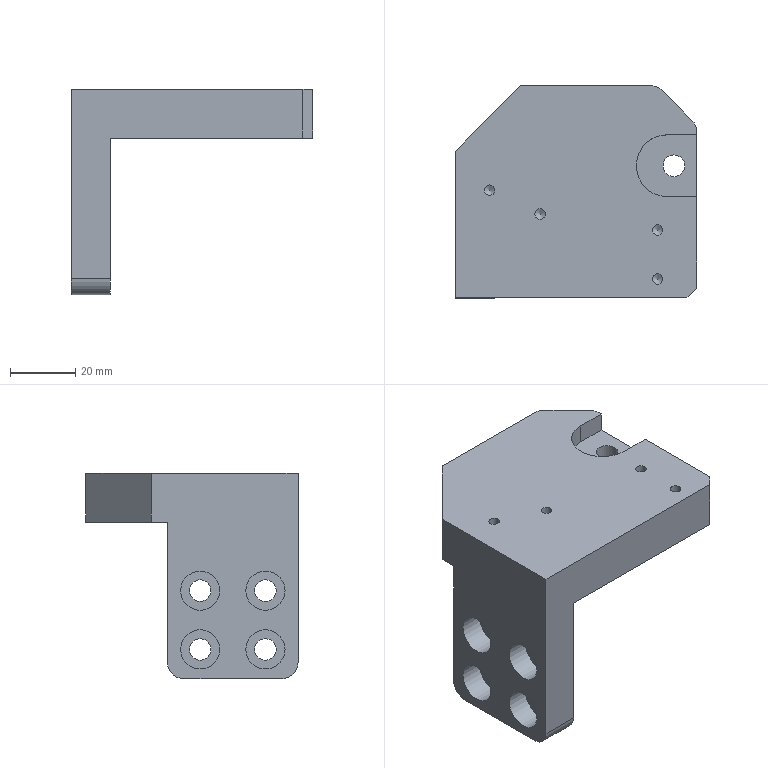Part | NX | 1 solid | 41 faces | box 74 x 65 x 63 mm | volume 84454 mm3 | plane 19 | cylinder 18 | cone 4 | commonest cylinder face diameters 3.242 x4 6.6 x4 10 x4 12 x4 6.647 x1 19 x1
STEP:
#1=CARTESIAN_POINT('',(-29.8,-5.8,-36.));
#2=VERTEX_POINT('',#1);
#3=CARTESIAN_POINT('',(-29.8,-2.5,-36.));
#4=DIRECTION('',(1.,0.,0.));
#5=DIRECTION('',(0.,-1.,0.));
#6=AXIS2_PLACEMENT_3D('',#3,#4,#5);
#7=CIRCLE('',#6,3.3);
#8=EDGE_CURVE('',#2,#2,#7,.T.);
#9=ORIENTED_EDGE('',*,*,#8,.T.);
#10=EDGE_LOOP('',(#9));
#11=FACE_BOUND('',#10,.T.);
#12=CARTESIAN_POINT('',(-29.8,-8.5,-36.));
#13=VERTEX_POINT('',#12);
#14=CARTESIAN_POINT('',(-29.8,-2.5,-36.));
#15=DIRECTION('',(-1.,0.,0.));
#16=DIRECTION('',(0.,-1.,0.));
#17=AXIS2_PLACEMENT_3D('',#14,#15,#16);
#18=CIRCLE('',#17,6.);
#19=EDGE_CURVE('',#13,#13,#18,.T.);
#20=ORIENTED_EDGE('',*,*,#19,.T.);
#21=EDGE_LOOP('',(#20));
#22=FACE_BOUND('',#21,.T.);
#23=CARTESIAN_POINT('',(-29.8,32.5,0.));
#24=DIRECTION('',(-1.,0.,0.));
#25=DIRECTION('',(0.,-1.,0.));
#26=AXIS2_PLACEMENT_3D('',#23,#24,#25);
#27=PLANE('',#26);
#28=ADVANCED_FACE('',(#11,#22),#27,.T.);
#29=CARTESIAN_POINT('',(-37.,-8.5,-36.));
#30=VERTEX_POINT('',#29);
#31=CARTESIAN_POINT('',(-37.,-2.5,-36.));
#32=DIRECTION('',(-1.,0.,0.));
#33=DIRECTION('',(0.,-1.,0.));
#34=AXIS2_PLACEMENT_3D('',#31,#32,#33);
#35=CIRCLE('',#34,6.);
#36=EDGE_CURVE('',#30,#30,#35,.T.);
#37=ORIENTED_EDGE('',*,*,#36,.T.);
#38=EDGE_LOOP('',(#37));
#39=FACE_BOUND('',#38,.T.);
#40=ORIENTED_EDGE('',*,*,#19,.F.);
#41=EDGE_LOOP('',(#40));
#42=FACE_BOUND('',#41,.T.);
#43=CARTESIAN_POINT('',(-33.4,-2.5,-36.));
#44=DIRECTION('',(-1.,0.,0.));
#45=DIRECTION('',(0.,-1.,0.));
#46=AXIS2_PLACEMENT_3D('',#43,#44,#45);
#47=CYLINDRICAL_SURFACE('',#46,6.);
#48=ADVANCED_FACE('',(#39,#42),#47,.F.);
#49=CARTESIAN_POINT('',(-29.8,-5.8,-54.));
#50=VERTEX_POINT('',#49);
#51=CARTESIAN_POINT('',(-29.8,-2.5,-54.));
#52=DIRECTION('',(1.,0.,0.));
#53=DIRECTION('',(0.,-1.,0.));
#54=AXIS2_PLACEMENT_3D('',#51,#52,#53);
#55=CIRCLE('',#54,3.3);
#56=EDGE_CURVE('',#50,#50,#55,.T.);
#57=ORIENTED_EDGE('',*,*,#56,.T.);
#58=EDGE_LOOP('',(#57));
#59=FACE_BOUND('',#58,.T.);
#60=CARTESIAN_POINT('',(-29.8,-8.5,-54.));
#61=VERTEX_POINT('',#60);
#62=CARTESIAN_POINT('',(-29.8,-2.5,-54.));
#63=DIRECTION('',(-1.,0.,0.));
#64=DIRECTION('',(0.,-1.,0.));
#65=AXIS2_PLACEMENT_3D('',#62,#63,#64);
#66=CIRCLE('',#65,6.);
#67=EDGE_CURVE('',#61,#61,#66,.T.);
#68=ORIENTED_EDGE('',*,*,#67,.T.);
#69=EDGE_LOOP('',(#68));
#70=FACE_BOUND('',#69,.T.);
#71=CARTESIAN_POINT('',(-29.8,32.5,0.));
#72=DIRECTION('',(-1.,0.,0.));
#73=DIRECTION('',(0.,-1.,0.));
#74=AXIS2_PLACEMENT_3D('',#71,#72,#73);
#75=PLANE('',#74);
#76=ADVANCED_FACE('',(#59,#70),#75,.T.);
#77=CARTESIAN_POINT('',(-37.,-8.5,-54.));
#78=VERTEX_POINT('',#77);
#79=CARTESIAN_POINT('',(-37.,-2.5,-54.));
#80=DIRECTION('',(-1.,0.,0.));
#81=DIRECTION('',(0.,-1.,0.));
#82=AXIS2_PLACEMENT_3D('',#79,#80,#81);
#83=CIRCLE('',#82,6.);
#84=EDGE_CURVE('',#78,#78,#83,.T.);
#85=ORIENTED_EDGE('',*,*,#84,.T.);
#86=EDGE_LOOP('',(#85));
#87=FACE_BOUND('',#86,.T.);
#88=ORIENTED_EDGE('',*,*,#67,.F.);
#89=EDGE_LOOP('',(#88));
#90=FACE_BOUND('',#89,.T.);
#91=CARTESIAN_POINT('',(-33.4,-2.5,-54.));
#92=DIRECTION('',(-1.,0.,0.));
#93=DIRECTION('',(0.,-1.,0.));
#94=AXIS2_PLACEMENT_3D('',#91,#92,#93);
#95=CYLINDRICAL_SURFACE('',#94,6.);
#96=ADVANCED_FACE('',(#87,#90),#95,.F.);
#97=CARTESIAN_POINT('',(-29.8,-25.8,-36.));
#98=VERTEX_POINT('',#97);
#99=CARTESIAN_POINT('',(-29.8,-22.5,-36.));
#100=DIRECTION('',(1.,0.,0.));
#101=DIRECTION('',(0.,-1.,0.));
#102=AXIS2_PLACEMENT_3D('',#99,#100,#101);
#103=CIRCLE('',#102,3.3);
#104=EDGE_CURVE('',#98,#98,#103,.T.);
#105=ORIENTED_EDGE('',*,*,#104,.T.);
#106=EDGE_LOOP('',(#105));
#107=FACE_BOUND('',#106,.T.);
#108=CARTESIAN_POINT('',(-29.8,-28.5,-36.));
#109=VERTEX_POINT('',#108);
#110=CARTESIAN_POINT('',(-29.8,-22.5,-36.));
#111=DIRECTION('',(-1.,0.,0.));
#112=DIRECTION('',(0.,-1.,0.));
#113=AXIS2_PLACEMENT_3D('',#110,#111,#112);
#114=CIRCLE('',#113,6.);
#115=EDGE_CURVE('',#109,#109,#114,.T.);
#116=ORIENTED_EDGE('',*,*,#115,.T.);
#117=EDGE_LOOP('',(#116));
#118=FACE_BOUND('',#117,.T.);
#119=CARTESIAN_POINT('',(-29.8,32.5,0.));
#120=DIRECTION('',(-1.,0.,0.));
#121=DIRECTION('',(0.,-1.,0.));
#122=AXIS2_PLACEMENT_3D('',#119,#120,#121);
#123=PLANE('',#122);
#124=ADVANCED_FACE('',(#107,#118),#123,.T.);
#125=CARTESIAN_POINT('',(-37.,-28.5,-36.));
#126=VERTEX_POINT('',#125);
#127=CARTESIAN_POINT('',(-37.,-22.5,-36.));
#128=DIRECTION('',(-1.,0.,0.));
#129=DIRECTION('',(0.,-1.,0.));
#130=AXIS2_PLACEMENT_3D('',#127,#128,#129);
#131=CIRCLE('',#130,6.);
#132=EDGE_CURVE('',#126,#126,#131,.T.);
#133=ORIENTED_EDGE('',*,*,#132,.T.);
#134=EDGE_LOOP('',(#133));
#135=FACE_BOUND('',#134,.T.);
#136=ORIENTED_EDGE('',*,*,#115,.F.);
#137=EDGE_LOOP('',(#136));
#138=FACE_BOUND('',#137,.T.);
#139=CARTESIAN_POINT('',(-33.4,-22.5,-36.));
#140=DIRECTION('',(-1.,0.,0.));
#141=DIRECTION('',(0.,-1.,0.));
#142=AXIS2_PLACEMENT_3D('',#139,#140,#141);
#143=CYLINDRICAL_SURFACE('',#142,6.);
#144=ADVANCED_FACE('',(#135,#138),#143,.F.);
#145=CARTESIAN_POINT('',(30.,4.676,-15.));
#146=VERTEX_POINT('',#145);
#147=CARTESIAN_POINT('',(30.,8.,-15.));
#148=DIRECTION('',(0.,0.,1.));
#149=DIRECTION('',(0.,-1.,0.));
#150=AXIS2_PLACEMENT_3D('',#147,#148,#149);
#151=CIRCLE('',#150,3.324);
#152=EDGE_CURVE('',#146,#146,#151,.T.);
#153=ORIENTED_EDGE('',*,*,#152,.F.);
#154=EDGE_LOOP('',(#153));
#155=FACE_BOUND('',#154,.T.);
#156=CARTESIAN_POINT('',(30.,4.676,-6.));
#157=VERTEX_POINT('',#156);
#158=CARTESIAN_POINT('',(30.,8.,-6.));
#159=DIRECTION('',(0.,0.,1.));
#160=DIRECTION('',(0.,-1.,0.));
#161=AXIS2_PLACEMENT_3D('',#158,#159,#160);
#162=CIRCLE('',#161,3.324);
#163=EDGE_CURVE('',#157,#157,#162,.T.);
#164=ORIENTED_EDGE('',*,*,#163,.T.);
#165=EDGE_LOOP('',(#164));
#166=FACE_BOUND('',#165,.T.);
#167=CARTESIAN_POINT('',(30.,8.,-6.));
#168=DIRECTION('',(0.,0.,-1.));
#169=DIRECTION('',(0.,-1.,0.));
#170=AXIS2_PLACEMENT_3D('',#167,#168,#169);
#171=CYLINDRICAL_SURFACE('',#170,3.324);
#172=ADVANCED_FACE('',(#155,#166),#171,.F.);
#173=CARTESIAN_POINT('',(-25.,-25.8,-54.));
#174=VERTEX_POINT('',#173);
#175=CARTESIAN_POINT('',(-25.,-22.5,-54.));
#176=DIRECTION('',(1.,0.,0.));
#177=DIRECTION('',(0.,-1.,0.));
#178=AXIS2_PLACEMENT_3D('',#175,#176,#177);
#179=CIRCLE('',#178,3.3);
#180=EDGE_CURVE('',#174,#174,#179,.T.);
#181=ORIENTED_EDGE('',*,*,#180,.T.);
#182=EDGE_LOOP('',(#181));
#183=FACE_BOUND('',#182,.T.);
#184=CARTESIAN_POINT('',(-29.8,-25.8,-54.));
#185=VERTEX_POINT('',#184);
#186=CARTESIAN_POINT('',(-29.8,-22.5,-54.));
#187=DIRECTION('',(-1.,0.,0.));
#188=DIRECTION('',(0.,-1.,0.));
#189=AXIS2_PLACEMENT_3D('',#186,#187,#188);
#190=CIRCLE('',#189,3.3);
#191=EDGE_CURVE('',#185,#185,#190,.T.);
#192=ORIENTED_EDGE('',*,*,#191,.T.);
#193=EDGE_LOOP('',(#192));
#194=FACE_BOUND('',#193,.T.);
#195=CARTESIAN_POINT('',(-57.5,-22.5,-54.));
#196=DIRECTION('',(1.,0.,0.));
#197=DIRECTION('',(0.,1.,0.));
#198=AXIS2_PLACEMENT_3D('',#195,#196,#197);
#199=CYLINDRICAL_SURFACE('',#198,3.3);
#200=ADVANCED_FACE('',(#183,#194),#199,.F.);
#201=CARTESIAN_POINT('',(-26.5,2.121,-10.));
#202=VERTEX_POINT('',#201);
#203=CARTESIAN_POINT('',(-26.5,0.5,-10.));
#204=DIRECTION('',(0.,0.,-1.));
#205=DIRECTION('',(0.,1.,0.));
#206=AXIS2_PLACEMENT_3D('',#203,#204,#205);
#207=CIRCLE('',#206,1.621);
#208=EDGE_CURVE('',#202,#202,#207,.T.);
#209=ORIENTED_EDGE('',*,*,#208,.F.);
#210=EDGE_LOOP('',(#209));
#211=FACE_BOUND('',#210,.T.);
#212=CARTESIAN_POINT('',(-26.5,0.5,-10.936));
#213=VERTEX_POINT('',#212);
#214=VERTEX_LOOP('',#213);
#215=FACE_BOUND('',#214,.T.);
#216=CARTESIAN_POINT('',(-26.5,0.5,-10.936));
#217=DIRECTION('',(0.,0.,1.));
#218=DIRECTION('',(0.,-1.,0.));
#219=AXIS2_PLACEMENT_3D('',#216,#217,#218);
#220=CONICAL_SURFACE('',#219,0.,1.047);
#221=ADVANCED_FACE('',(#211,#215),#220,.F.);
#222=CARTESIAN_POINT('',(-11.,-5.179,-10.));
#223=VERTEX_POINT('',#222);
#224=CARTESIAN_POINT('',(-11.,-6.8,-10.));
#225=DIRECTION('',(0.,0.,-1.));
#226=DIRECTION('',(0.,1.,0.));
#227=AXIS2_PLACEMENT_3D('',#224,#225,#226);
#228=CIRCLE('',#227,1.621);
#229=EDGE_CURVE('',#223,#223,#228,.T.);
#230=ORIENTED_EDGE('',*,*,#229,.F.);
#231=EDGE_LOOP('',(#230));
#232=FACE_BOUND('',#231,.T.);
#233=CARTESIAN_POINT('',(-11.,-6.8,-10.936));
#234=VERTEX_POINT('',#233);
#235=VERTEX_LOOP('',#234);
#236=FACE_BOUND('',#235,.T.);
#237=CARTESIAN_POINT('',(-11.,-6.8,-10.936));
#238=DIRECTION('',(0.,0.,1.));
#239=DIRECTION('',(0.,-1.,0.));
#240=AXIS2_PLACEMENT_3D('',#237,#238,#239);
#241=CONICAL_SURFACE('',#240,0.,1.047);
#242=ADVANCED_FACE('',(#232,#236),#241,.F.);
#243=CARTESIAN_POINT('',(25.,-10.079,-10.));
#244=VERTEX_POINT('',#243);
#245=CARTESIAN_POINT('',(25.,-11.7,-10.));
#246=DIRECTION('',(0.,0.,-1.));
#247=DIRECTION('',(0.,1.,0.));
#248=AXIS2_PLACEMENT_3D('',#245,#246,#247);
#249=CIRCLE('',#248,1.621);
#250=EDGE_CURVE('',#244,#244,#249,.T.);
#251=ORIENTED_EDGE('',*,*,#250,.F.);
#252=EDGE_LOOP('',(#251));
#253=FACE_BOUND('',#252,.T.);
#254=CARTESIAN_POINT('',(25.,-11.7,-10.936));
#255=VERTEX_POINT('',#254);
#256=VERTEX_LOOP('',#255);
#257=FACE_BOUND('',#256,.T.);
#258=CARTESIAN_POINT('',(25.,-11.7,-10.936));
#259=DIRECTION('',(0.,0.,1.));
#260=DIRECTION('',(0.,-1.,0.));
#261=AXIS2_PLACEMENT_3D('',#258,#259,#260);
#262=CONICAL_SURFACE('',#261,0.,1.047);
#263=ADVANCED_FACE('',(#253,#257),#262,.F.);
#264=ORIENTED_EDGE('',*,*,#163,.F.);
#265=EDGE_LOOP('',(#264));
#266=FACE_BOUND('',#265,.T.);
#267=CARTESIAN_POINT('',(28.,17.5,-6.));
#268=VERTEX_POINT('',#267);
#269=CARTESIAN_POINT('',(37.,17.5,-6.));
#270=VERTEX_POINT('',#269);
#271=CARTESIAN_POINT('',(32.5,17.5,-6.));
#272=DIRECTION('',(1.,0.,0.));
#273=VECTOR('',#272,1000.);
#274=LINE('',#271,#273);
#275=EDGE_CURVE('',#268,#270,#274,.T.);
#276=ORIENTED_EDGE('',*,*,#275,.F.);
#277=CARTESIAN_POINT('',(28.,-1.5,-6.));
#278=VERTEX_POINT('',#277);
#279=CARTESIAN_POINT('',(28.,8.,-6.));
#280=DIRECTION('',(0.,0.,1.));
#281=DIRECTION('',(0.,-1.,0.));
#282=AXIS2_PLACEMENT_3D('',#279,#280,#281);
#283=CIRCLE('',#282,9.5);
#284=EDGE_CURVE('',#268,#278,#283,.T.);
#285=ORIENTED_EDGE('',*,*,#284,.T.);
#286=CARTESIAN_POINT('',(37.,-1.5,-6.));
#287=VERTEX_POINT('',#286);
#288=CARTESIAN_POINT('',(32.5,-1.5,-6.));
#289=DIRECTION('',(-1.,0.,0.));
#290=VECTOR('',#289,1000.);
#291=LINE('',#288,#290);
#292=EDGE_CURVE('',#287,#278,#291,.T.);
#293=ORIENTED_EDGE('',*,*,#292,.F.);
#294=CARTESIAN_POINT('',(37.,8.,-6.));
#295=DIRECTION('',(0.,-1.,0.));
#296=VECTOR('',#295,1000.);
#297=LINE('',#294,#296);
#298=EDGE_CURVE('',#270,#287,#297,.T.);
#299=ORIENTED_EDGE('',*,*,#298,.F.);
#300=EDGE_LOOP('',(#276,#285,#293,#299));
#301=FACE_BOUND('',#300,.T.);
#302=CARTESIAN_POINT('',(-37.,32.5,-6.));
#303=DIRECTION('',(0.,0.,1.));
#304=DIRECTION('',(0.,-1.,0.));
#305=AXIS2_PLACEMENT_3D('',#302,#303,#304);
#306=PLANE('',#305);
#307=ADVANCED_FACE('',(#266,#301),#306,.T.);
#308=CARTESIAN_POINT('',(-25.,-5.8,-36.));
#309=VERTEX_POINT('',#308);
#310=CARTESIAN_POINT('',(-25.,-2.5,-36.));
#311=DIRECTION('',(1.,0.,0.));
#312=DIRECTION('',(0.,-1.,0.));
#313=AXIS2_PLACEMENT_3D('',#310,#311,#312);
#314=CIRCLE('',#313,3.3);
#315=EDGE_CURVE('',#309,#309,#314,.T.);
#316=ORIENTED_EDGE('',*,*,#315,.T.);
#317=EDGE_LOOP('',(#316));
#318=FACE_BOUND('',#317,.T.);
#319=ORIENTED_EDGE('',*,*,#8,.F.);
#320=EDGE_LOOP('',(#319));
#321=FACE_BOUND('',#320,.T.);
#322=CARTESIAN_POINT('',(-57.5,-2.5,-36.));
#323=DIRECTION('',(1.,0.,0.));
#324=DIRECTION('',(0.,1.,0.));
#325=AXIS2_PLACEMENT_3D('',#322,#323,#324);
#326=CYLINDRICAL_SURFACE('',#325,3.3);
#327=ADVANCED_FACE('',(#318,#321),#326,.F.);
#328=CARTESIAN_POINT('',(-25.,-5.8,-54.));
#329=VERTEX_POINT('',#328);
#330=CARTESIAN_POINT('',(-25.,-2.5,-54.));
#331=DIRECTION('',(1.,0.,0.));
#332=DIRECTION('',(0.,-1.,0.));
#333=AXIS2_PLACEMENT_3D('',#330,#331,#332);
#334=CIRCLE('',#333,3.3);
#335=EDGE_CURVE('',#329,#329,#334,.T.);
#336=ORIENTED_EDGE('',*,*,#335,.T.);
#337=EDGE_LOOP('',(#336));
#338=FACE_BOUND('',#337,.T.);
#339=ORIENTED_EDGE('',*,*,#56,.F.);
#340=EDGE_LOOP('',(#339));
#341=FACE_BOUND('',#340,.T.);
#342=CARTESIAN_POINT('',(-57.5,-2.5,-54.));
#343=DIRECTION('',(1.,0.,0.));
#344=DIRECTION('',(0.,1.,0.));
#345=AXIS2_PLACEMENT_3D('',#342,#343,#344);
#346=CYLINDRICAL_SURFACE('',#345,3.3);
#347=ADVANCED_FACE('',(#338,#341),#346,.F.);
#348=CARTESIAN_POINT('',(-25.,-25.8,-36.));
#349=VERTEX_POINT('',#348);
#350=CARTESIAN_POINT('',(-25.,-22.5,-36.));
#351=DIRECTION('',(1.,0.,0.));
#352=DIRECTION('',(0.,-1.,0.));
#353=AXIS2_PLACEMENT_3D('',#350,#351,#352);
#354=CIRCLE('',#353,3.3);
#355=EDGE_CURVE('',#349,#349,#354,.T.);
#356=ORIENTED_EDGE('',*,*,#355,.T.);
#357=EDGE_LOOP('',(#356));
#358=FACE_BOUND('',#357,.T.);
#359=ORIENTED_EDGE('',*,*,#104,.F.);
#360=EDGE_LOOP('',(#359));
#361=FACE_BOUND('',#360,.T.);
#362=CARTESIAN_POINT('',(-57.5,-22.5,-36.));
#363=DIRECTION('',(1.,0.,0.));
#364=DIRECTION('',(0.,1.,0.));
#365=AXIS2_PLACEMENT_3D('',#362,#363,#364);
#366=CYLINDRICAL_SURFACE('',#365,3.3);
#367=ADVANCED_FACE('',(#358,#361),#366,.F.);
#368=CARTESIAN_POINT('',(-25.,-27.5,-63.));
#369=VERTEX_POINT('',#368);
#370=CARTESIAN_POINT('',(-37.,-27.5,-63.));
#371=VERTEX_POINT('',#370);
#372=CARTESIAN_POINT('',(0.,-27.5,-63.));
#373=DIRECTION('',(-1.,0.,0.));
#374=VECTOR('',#373,1000.);
#375=LINE('',#372,#374);
#376=EDGE_CURVE('',#369,#371,#375,.T.);
#377=ORIENTED_EDGE('',*,*,#376,.T.);
#378=CARTESIAN_POINT('',(-37.,2.5,-63.));
#379=VERTEX_POINT('',#378);
#380=CARTESIAN_POINT('',(-37.,-12.5,-63.));
#381=DIRECTION('',(0.,-1.,0.));
#382=VECTOR('',#381,1000.);
#383=LINE('',#380,#382);
#384=EDGE_CURVE('',#379,#371,#383,.T.);
#385=ORIENTED_EDGE('',*,*,#384,.F.);
#386=CARTESIAN_POINT('',(-25.,2.5,-63.));
#387=VERTEX_POINT('',#386);
#388=CARTESIAN_POINT('',(-31.,2.5,-63.));
#389=DIRECTION('',(-1.,0.,0.));
#390=VECTOR('',#389,1000.);
#391=LINE('',#388,#390);
#392=EDGE_CURVE('',#387,#379,#391,.T.);
#393=ORIENTED_EDGE('',*,*,#392,.F.);
#394=CARTESIAN_POINT('',(-25.,-12.5,-63.));
#395=DIRECTION('',(0.,-1.,0.));
#396=VECTOR('',#395,1000.);
#397=LINE('',#394,#396);
#398=EDGE_CURVE('',#387,#369,#397,.T.);
#399=ORIENTED_EDGE('',*,*,#398,.T.);
#400=EDGE_LOOP('',(#377,#385,#393,#399));
#401=FACE_BOUND('',#400,.T.);
#402=CARTESIAN_POINT('',(-25.,32.5,-63.));
#403=DIRECTION('',(0.,0.,1.));
#404=DIRECTION('',(-1.,0.,0.));
#405=AXIS2_PLACEMENT_3D('',#402,#403,#404);
#406=PLANE('',#405);
#407=ADVANCED_FACE('',(#401),#406,.F.);
#408=CARTESIAN_POINT('',(-37.,7.5,-58.));
#409=VERTEX_POINT('',#408);
#410=CARTESIAN_POINT('',(-37.,2.5,-58.));
#411=DIRECTION('',(-1.,0.,0.));
#412=DIRECTION('',(0.,-1.,0.));
#413=AXIS2_PLACEMENT_3D('',#410,#411,#412);
#414=CIRCLE('',#413,5.);
#415=EDGE_CURVE('',#409,#379,#414,.T.);
#416=ORIENTED_EDGE('',*,*,#415,.F.);
#417=CARTESIAN_POINT('',(-25.,7.5,-58.));
#418=VERTEX_POINT('',#417);
#419=CARTESIAN_POINT('',(-31.,7.5,-58.));
#420=DIRECTION('',(-1.,0.,0.));
#421=VECTOR('',#420,1000.);
#422=LINE('',#419,#421);
#423=EDGE_CURVE('',#418,#409,#422,.T.);
#424=ORIENTED_EDGE('',*,*,#423,.F.);
#425=CARTESIAN_POINT('',(-25.,2.5,-58.));
#426=DIRECTION('',(1.,0.,0.));
#427=DIRECTION('',(0.,-1.,0.));
#428=AXIS2_PLACEMENT_3D('',#425,#426,#427);
#429=CIRCLE('',#428,5.);
#430=EDGE_CURVE('',#387,#418,#429,.T.);
#431=ORIENTED_EDGE('',*,*,#430,.F.);
#432=ORIENTED_EDGE('',*,*,#392,.T.);
#433=EDGE_LOOP('',(#416,#424,#431,#432));
#434=FACE_BOUND('',#433,.T.);
#435=CARTESIAN_POINT('',(-31.,2.5,-58.));
#436=DIRECTION('',(-1.,0.,0.));
#437=DIRECTION('',(0.,1.,0.));
#438=AXIS2_PLACEMENT_3D('',#435,#436,#437);
#439=CYLINDRICAL_SURFACE('',#438,5.);
#440=ADVANCED_FACE('',(#434),#439,.T.);
#441=ORIENTED_EDGE('',*,*,#423,.T.);
#442=CARTESIAN_POINT('',(-37.,7.5,-15.));
#443=VERTEX_POINT('',#442);
#444=CARTESIAN_POINT('',(-37.,7.5,-36.5));
#445=DIRECTION('',(0.,0.,1.));
#446=VECTOR('',#445,1000.);
#447=LINE('',#444,#446);
#448=EDGE_CURVE('',#409,#443,#447,.T.);
#449=ORIENTED_EDGE('',*,*,#448,.T.);
#450=CARTESIAN_POINT('',(-25.,7.5,-15.));
#451=VERTEX_POINT('',#450);
#452=CARTESIAN_POINT('',(-31.,7.5,-15.));
#453=DIRECTION('',(-1.,0.,0.));
#454=VECTOR('',#453,1000.);
#455=LINE('',#452,#454);
#456=EDGE_CURVE('',#451,#443,#455,.T.);
#457=ORIENTED_EDGE('',*,*,#456,.F.);
#458=CARTESIAN_POINT('',(-25.,7.5,-36.5));
#459=DIRECTION('',(0.,0.,1.));
#460=VECTOR('',#459,1000.);
#461=LINE('',#458,#460);
#462=EDGE_CURVE('',#418,#451,#461,.T.);
#463=ORIENTED_EDGE('',*,*,#462,.F.);
#464=EDGE_LOOP('',(#441,#449,#457,#463));
#465=FACE_BOUND('',#464,.T.);
#466=CARTESIAN_POINT('',(-25.,7.5,-63.));
#467=DIRECTION('',(0.,-1.,0.));
#468=DIRECTION('',(0.,0.,1.));
#469=AXIS2_PLACEMENT_3D('',#466,#467,#468);
#470=PLANE('',#469);
#471=ADVANCED_FACE('',(#465),#470,.F.);
#472=ORIENTED_EDGE('',*,*,#152,.T.);
#473=EDGE_LOOP('',(#472));
#474=FACE_BOUND('',#473,.T.);
#475=CARTESIAN_POINT('',(37.,-29.5,-15.));
#476=VERTEX_POINT('',#475);
#477=CARTESIAN_POINT('',(34.,-32.5,-15.));
#478=VERTEX_POINT('',#477);
#479=CARTESIAN_POINT('',(35.5,-31.,-15.));
#480=DIRECTION('',(-0.7071,-0.7071,0.));
#481=VECTOR('',#480,1000.);
#482=LINE('',#479,#481);
#483=EDGE_CURVE('',#476,#478,#482,.T.);
#484=ORIENTED_EDGE('',*,*,#483,.T.);
#485=CARTESIAN_POINT('',(-25.,-32.5,-15.));
#486=VERTEX_POINT('',#485);
#487=CARTESIAN_POINT('',(4.5,-32.5,-15.));
#488=DIRECTION('',(-1.,0.,0.));
#489=VECTOR('',#488,1000.);
#490=LINE('',#487,#489);
#491=EDGE_CURVE('',#478,#486,#490,.T.);
#492=ORIENTED_EDGE('',*,*,#491,.T.);
#493=CARTESIAN_POINT('',(-25.,-12.5,-15.));
#494=DIRECTION('',(0.,-1.,0.));
#495=VECTOR('',#494,1000.);
#496=LINE('',#493,#495);
#497=EDGE_CURVE('',#451,#486,#496,.T.);
#498=ORIENTED_EDGE('',*,*,#497,.F.);
#499=ORIENTED_EDGE('',*,*,#456,.T.);
#500=CARTESIAN_POINT('',(-37.,12.5,-15.));
#501=VERTEX_POINT('',#500);
#502=CARTESIAN_POINT('',(-37.,10.,-15.));
#503=DIRECTION('',(0.,-1.,0.));
#504=VECTOR('',#503,1000.);
#505=LINE('',#502,#504);
#506=EDGE_CURVE('',#501,#443,#505,.T.);
#507=ORIENTED_EDGE('',*,*,#506,.F.);
#508=CARTESIAN_POINT('',(-17.,32.5,-15.));
#509=VERTEX_POINT('',#508);
#510=CARTESIAN_POINT('',(-27.,22.5,-15.));
#511=DIRECTION('',(-0.7071,-0.7071,0.));
#512=VECTOR('',#511,1000.);
#513=LINE('',#510,#512);
#514=EDGE_CURVE('',#509,#501,#513,.T.);
#515=ORIENTED_EDGE('',*,*,#514,.F.);
#516=CARTESIAN_POINT('',(22.929,32.5,-15.));
#517=VERTEX_POINT('',#516);
#518=CARTESIAN_POINT('',(2.964,32.5,-15.));
#519=DIRECTION('',(-1.,0.,0.));
#520=VECTOR('',#519,1000.);
#521=LINE('',#518,#520);
#522=EDGE_CURVE('',#517,#509,#521,.T.);
#523=ORIENTED_EDGE('',*,*,#522,.F.);
#524=CARTESIAN_POINT('',(26.464,31.036,-15.));
#525=VERTEX_POINT('',#524);
#526=CARTESIAN_POINT('',(22.929,27.5,-15.));
#527=DIRECTION('',(0.,0.,1.));
#528=DIRECTION('',(0.,-1.,0.));
#529=AXIS2_PLACEMENT_3D('',#526,#527,#528);
#530=CIRCLE('',#529,5.);
#531=EDGE_CURVE('',#525,#517,#530,.T.);
#532=ORIENTED_EDGE('',*,*,#531,.F.);
#533=CARTESIAN_POINT('',(35.536,21.964,-15.));
#534=VERTEX_POINT('',#533);
#535=CARTESIAN_POINT('',(31.,26.5,-15.));
#536=DIRECTION('',(0.7071,-0.7071,0.));
#537=VECTOR('',#536,1000.);
#538=LINE('',#535,#537);
#539=EDGE_CURVE('',#525,#534,#538,.T.);
#540=ORIENTED_EDGE('',*,*,#539,.T.);
#541=CARTESIAN_POINT('',(37.,18.429,-15.));
#542=VERTEX_POINT('',#541);
#543=CARTESIAN_POINT('',(32.,18.429,-15.));
#544=DIRECTION('',(0.,0.,1.));
#545=DIRECTION('',(0.,-1.,0.));
#546=AXIS2_PLACEMENT_3D('',#543,#544,#545);
#547=CIRCLE('',#546,5.);
#548=EDGE_CURVE('',#542,#534,#547,.T.);
#549=ORIENTED_EDGE('',*,*,#548,.F.);
#550=CARTESIAN_POINT('',(37.,-5.536,-15.));
#551=DIRECTION('',(0.,-1.,0.));
#552=VECTOR('',#551,1000.);
#553=LINE('',#550,#552);
#554=EDGE_CURVE('',#542,#476,#553,.T.);
#555=ORIENTED_EDGE('',*,*,#554,.T.);
#556=EDGE_LOOP('',(#484,#492,#498,#499,#507,#515,#523,#532,#540,#549,#555));
#557=FACE_BOUND('',#556,.T.);
#558=CARTESIAN_POINT('',(37.,32.5,-15.));
#559=DIRECTION('',(0.,0.,1.));
#560=DIRECTION('',(-1.,0.,0.));
#561=AXIS2_PLACEMENT_3D('',#558,#559,#560);
#562=PLANE('',#561);
#563=ADVANCED_FACE('',(#474,#557),#562,.F.);
#564=ORIENTED_EDGE('',*,*,#315,.F.);
#565=EDGE_LOOP('',(#564));
#566=FACE_BOUND('',#565,.T.);
#567=ORIENTED_EDGE('',*,*,#335,.F.);
#568=EDGE_LOOP('',(#567));
#569=FACE_BOUND('',#568,.T.);
#570=ORIENTED_EDGE('',*,*,#355,.F.);
#571=EDGE_LOOP('',(#570));
#572=FACE_BOUND('',#571,.T.);
#573=ORIENTED_EDGE('',*,*,#180,.F.);
#574=EDGE_LOOP('',(#573));
#575=FACE_BOUND('',#574,.T.);
#576=ORIENTED_EDGE('',*,*,#398,.F.);
#577=ORIENTED_EDGE('',*,*,#430,.T.);
#578=ORIENTED_EDGE('',*,*,#462,.T.);
#579=ORIENTED_EDGE('',*,*,#497,.T.);
#580=CARTESIAN_POINT('',(-25.,-32.5,-58.));
#581=VERTEX_POINT('',#580);
#582=CARTESIAN_POINT('',(-25.,-32.5,-36.5));
#583=DIRECTION('',(0.,0.,1.));
#584=VECTOR('',#583,1000.);
#585=LINE('',#582,#584);
#586=EDGE_CURVE('',#581,#486,#585,.T.);
#587=ORIENTED_EDGE('',*,*,#586,.F.);
#588=CARTESIAN_POINT('',(-25.,-27.5,-58.));
#589=DIRECTION('',(-1.,0.,0.));
#590=DIRECTION('',(0.,-1.,0.));
#591=AXIS2_PLACEMENT_3D('',#588,#589,#590);
#592=CIRCLE('',#591,5.);
#593=EDGE_CURVE('',#369,#581,#592,.T.);
#594=ORIENTED_EDGE('',*,*,#593,.F.);
#595=EDGE_LOOP('',(#576,#577,#578,#579,#587,#594));
#596=FACE_BOUND('',#595,.T.);
#597=CARTESIAN_POINT('',(-25.,32.5,-63.));
#598=DIRECTION('',(1.,0.,0.));
#599=DIRECTION('',(0.,0.,1.));
#600=AXIS2_PLACEMENT_3D('',#597,#598,#599);
#601=PLANE('',#600);
#602=ADVANCED_FACE('',(#566,#569,#572,#575,#596),#601,.T.);
#603=ORIENTED_EDGE('',*,*,#593,.T.);
#604=CARTESIAN_POINT('',(-37.,-32.5,-58.));
#605=VERTEX_POINT('',#604);
#606=CARTESIAN_POINT('',(-31.,-32.5,-58.));
#607=DIRECTION('',(-1.,0.,0.));
#608=VECTOR('',#607,1000.);
#609=LINE('',#606,#608);
#610=EDGE_CURVE('',#581,#605,#609,.T.);
#611=ORIENTED_EDGE('',*,*,#610,.T.);
#612=CARTESIAN_POINT('',(-37.,-27.5,-58.));
#613=DIRECTION('',(-1.,0.,0.));
#614=DIRECTION('',(0.,-1.,0.));
#615=AXIS2_PLACEMENT_3D('',#612,#613,#614);
#616=CIRCLE('',#615,5.);
#617=EDGE_CURVE('',#371,#605,#616,.T.);
#618=ORIENTED_EDGE('',*,*,#617,.F.);
#619=ORIENTED_EDGE('',*,*,#376,.F.);
#620=EDGE_LOOP('',(#603,#611,#618,#619));
#621=FACE_BOUND('',#620,.T.);
#622=CARTESIAN_POINT('',(0.,-27.5,-58.));
#623=DIRECTION('',(-1.,0.,0.));
#624=DIRECTION('',(0.,0.,-1.));
#625=AXIS2_PLACEMENT_3D('',#622,#623,#624);
#626=CYLINDRICAL_SURFACE('',#625,5.);
#627=ADVANCED_FACE('',(#621),#626,.T.);
#628=ORIENTED_EDGE('',*,*,#208,.T.);
#629=EDGE_LOOP('',(#628));
#630=FACE_BOUND('',#629,.T.);
#631=CARTESIAN_POINT('',(-26.5,2.121,0.));
#632=VERTEX_POINT('',#631);
#633=CARTESIAN_POINT('',(-26.5,0.5,0.));
#634=DIRECTION('',(0.,0.,-1.));
#635=DIRECTION('',(0.,1.,0.));
#636=AXIS2_PLACEMENT_3D('',#633,#634,#635);
#637=CIRCLE('',#636,1.621);
#638=EDGE_CURVE('',#632,#632,#637,.T.);
#639=ORIENTED_EDGE('',*,*,#638,.F.);
#640=EDGE_LOOP('',(#639));
#641=FACE_BOUND('',#640,.T.);
#642=CARTESIAN_POINT('',(-26.5,0.5,0.));
#643=DIRECTION('',(0.,0.,-1.));
#644=DIRECTION('',(0.,-1.,0.));
#645=AXIS2_PLACEMENT_3D('',#642,#643,#644);
#646=CYLINDRICAL_SURFACE('',#645,1.621);
#647=ADVANCED_FACE('',(#630,#641),#646,.F.);
#648=ORIENTED_EDGE('',*,*,#229,.T.);
#649=EDGE_LOOP('',(#648));
#650=FACE_BOUND('',#649,.T.);
#651=CARTESIAN_POINT('',(-11.,-5.179,0.));
#652=VERTEX_POINT('',#651);
#653=CARTESIAN_POINT('',(-11.,-6.8,0.));
#654=DIRECTION('',(0.,0.,-1.));
#655=DIRECTION('',(0.,1.,0.));
#656=AXIS2_PLACEMENT_3D('',#653,#654,#655);
#657=CIRCLE('',#656,1.621);
#658=EDGE_CURVE('',#652,#652,#657,.T.);
#659=ORIENTED_EDGE('',*,*,#658,.F.);
#660=EDGE_LOOP('',(#659));
#661=FACE_BOUND('',#660,.T.);
#662=CARTESIAN_POINT('',(-11.,-6.8,0.));
#663=DIRECTION('',(0.,0.,-1.));
#664=DIRECTION('',(0.,-1.,0.));
#665=AXIS2_PLACEMENT_3D('',#662,#663,#664);
#666=CYLINDRICAL_SURFACE('',#665,1.621);
#667=ADVANCED_FACE('',(#650,#661),#666,.F.);
#668=ORIENTED_EDGE('',*,*,#250,.T.);
#669=EDGE_LOOP('',(#668));
#670=FACE_BOUND('',#669,.T.);
#671=CARTESIAN_POINT('',(25.,-10.079,0.));
#672=VERTEX_POINT('',#671);
#673=CARTESIAN_POINT('',(25.,-11.7,0.));
#674=DIRECTION('',(0.,0.,-1.));
#675=DIRECTION('',(0.,1.,0.));
#676=AXIS2_PLACEMENT_3D('',#673,#674,#675);
#677=CIRCLE('',#676,1.621);
#678=EDGE_CURVE('',#672,#672,#677,.T.);
#679=ORIENTED_EDGE('',*,*,#678,.F.);
#680=EDGE_LOOP('',(#679));
#681=FACE_BOUND('',#680,.T.);
#682=CARTESIAN_POINT('',(25.,-11.7,0.));
#683=DIRECTION('',(0.,0.,-1.));
#684=DIRECTION('',(0.,-1.,0.));
#685=AXIS2_PLACEMENT_3D('',#682,#683,#684);
#686=CYLINDRICAL_SURFACE('',#685,1.621);
#687=ADVANCED_FACE('',(#670,#681),#686,.F.);
#688=CARTESIAN_POINT('',(34.,-32.5,0.));
#689=VERTEX_POINT('',#688);
#690=CARTESIAN_POINT('',(37.,-29.5,0.));
#691=VERTEX_POINT('',#690);
#692=CARTESIAN_POINT('',(35.5,-31.,0.));
#693=DIRECTION('',(0.7071,0.7071,0.));
#694=VECTOR('',#693,1000.);
#695=LINE('',#692,#694);
#696=EDGE_CURVE('',#689,#691,#695,.T.);
#697=ORIENTED_EDGE('',*,*,#696,.F.);
#698=CARTESIAN_POINT('',(34.,-32.5,-7.5));
#699=DIRECTION('',(0.,0.,1.));
#700=VECTOR('',#699,1000.);
#701=LINE('',#698,#700);
#702=EDGE_CURVE('',#478,#689,#701,.T.);
#703=ORIENTED_EDGE('',*,*,#702,.F.);
#704=ORIENTED_EDGE('',*,*,#483,.F.);
#705=CARTESIAN_POINT('',(37.,-29.5,-7.5));
#706=DIRECTION('',(0.,0.,1.));
#707=VECTOR('',#706,1000.);
#708=LINE('',#705,#707);
#709=EDGE_CURVE('',#476,#691,#708,.T.);
#710=ORIENTED_EDGE('',*,*,#709,.T.);
#711=EDGE_LOOP('',(#697,#703,#704,#710));
#712=FACE_BOUND('',#711,.T.);
#713=CARTESIAN_POINT('',(37.,-29.5,-29.));
#714=DIRECTION('',(0.7071,-0.7071,0.));
#715=DIRECTION('',(0.,0.,1.));
#716=AXIS2_PLACEMENT_3D('',#713,#714,#715);
#717=PLANE('',#716);
#718=ADVANCED_FACE('',(#712),#717,.T.);
#719=CARTESIAN_POINT('',(37.,-1.5,0.));
#720=VERTEX_POINT('',#719);
#721=CARTESIAN_POINT('',(37.,-1.5,-3.));
#722=DIRECTION('',(0.,0.,-1.));
#723=VECTOR('',#722,1000.);
#724=LINE('',#721,#723);
#725=EDGE_CURVE('',#720,#287,#724,.T.);
#726=ORIENTED_EDGE('',*,*,#725,.T.);
#727=ORIENTED_EDGE('',*,*,#292,.T.);
#728=CARTESIAN_POINT('',(28.,-1.5,0.));
#729=VERTEX_POINT('',#728);
#730=CARTESIAN_POINT('',(28.,-1.5,-3.));
#731=DIRECTION('',(0.,0.,1.));
#732=VECTOR('',#731,1000.);
#733=LINE('',#730,#732);
#734=EDGE_CURVE('',#278,#729,#733,.T.);
#735=ORIENTED_EDGE('',*,*,#734,.T.);
#736=CARTESIAN_POINT('',(32.5,-1.5,0.));
#737=DIRECTION('',(-1.,0.,0.));
#738=VECTOR('',#737,1000.);
#739=LINE('',#736,#738);
#740=EDGE_CURVE('',#720,#729,#739,.T.);
#741=ORIENTED_EDGE('',*,*,#740,.F.);
#742=EDGE_LOOP('',(#726,#727,#735,#741));
#743=FACE_BOUND('',#742,.T.);
#744=CARTESIAN_POINT('',(47.409,-1.5,0.));
#745=DIRECTION('',(0.,-1.,0.));
#746=DIRECTION('',(-1.,0.,0.));
#747=AXIS2_PLACEMENT_3D('',#744,#745,#746);
#748=PLANE('',#747);
#749=ADVANCED_FACE('',(#743),#748,.F.);
#750=CARTESIAN_POINT('',(28.,17.5,0.));
#751=VERTEX_POINT('',#750);
#752=CARTESIAN_POINT('',(28.,17.5,-3.));
#753=DIRECTION('',(0.,0.,-1.));
#754=VECTOR('',#753,1000.);
#755=LINE('',#752,#754);
#756=EDGE_CURVE('',#751,#268,#755,.T.);
#757=ORIENTED_EDGE('',*,*,#756,.F.);
#758=CARTESIAN_POINT('',(28.,8.,0.));
#759=DIRECTION('',(0.,0.,-1.));
#760=DIRECTION('',(0.,1.,0.));
#761=AXIS2_PLACEMENT_3D('',#758,#759,#760);
#762=CIRCLE('',#761,9.5);
#763=EDGE_CURVE('',#729,#751,#762,.T.);
#764=ORIENTED_EDGE('',*,*,#763,.F.);
#765=ORIENTED_EDGE('',*,*,#734,.F.);
#766=ORIENTED_EDGE('',*,*,#284,.F.);
#767=EDGE_LOOP('',(#757,#764,#765,#766));
#768=FACE_BOUND('',#767,.T.);
#769=CARTESIAN_POINT('',(28.,8.,-3.));
#770=DIRECTION('',(0.,0.,1.));
#771=DIRECTION('',(0.,1.,0.));
#772=AXIS2_PLACEMENT_3D('',#769,#770,#771);
#773=CYLINDRICAL_SURFACE('',#772,9.5);
#774=ADVANCED_FACE('',(#768),#773,.F.);
#775=CARTESIAN_POINT('',(37.,17.5,0.));
#776=VERTEX_POINT('',#775);
#777=CARTESIAN_POINT('',(37.,17.5,-3.));
#778=DIRECTION('',(0.,0.,-1.));
#779=VECTOR('',#778,1000.);
#780=LINE('',#777,#779);
#781=EDGE_CURVE('',#776,#270,#780,.T.);
#782=ORIENTED_EDGE('',*,*,#781,.F.);
#783=CARTESIAN_POINT('',(32.5,17.5,0.));
#784=DIRECTION('',(1.,0.,0.));
#785=VECTOR('',#784,1000.);
#786=LINE('',#783,#785);
#787=EDGE_CURVE('',#751,#776,#786,.T.);
#788=ORIENTED_EDGE('',*,*,#787,.F.);
#789=ORIENTED_EDGE('',*,*,#756,.T.);
#790=ORIENTED_EDGE('',*,*,#275,.T.);
#791=EDGE_LOOP('',(#782,#788,#789,#790));
#792=FACE_BOUND('',#791,.T.);
#793=CARTESIAN_POINT('',(28.,17.5,0.));
#794=DIRECTION('',(0.,1.,0.));
#795=DIRECTION('',(1.,0.,0.));
#796=AXIS2_PLACEMENT_3D('',#793,#794,#795);
#797=PLANE('',#796);
#798=ADVANCED_FACE('',(#792),#797,.F.);
#799=ORIENTED_EDGE('',*,*,#554,.F.);
#800=CARTESIAN_POINT('',(37.,18.429,0.));
#801=VERTEX_POINT('',#800);
#802=CARTESIAN_POINT('',(37.,18.429,-7.5));
#803=DIRECTION('',(0.,0.,1.));
#804=VECTOR('',#803,1000.);
#805=LINE('',#802,#804);
#806=EDGE_CURVE('',#542,#801,#805,.T.);
#807=ORIENTED_EDGE('',*,*,#806,.T.);
#808=CARTESIAN_POINT('',(37.,17.964,0.));
#809=DIRECTION('',(0.,-1.,0.));
#810=VECTOR('',#809,1000.);
#811=LINE('',#808,#810);
#812=EDGE_CURVE('',#801,#776,#811,.T.);
#813=ORIENTED_EDGE('',*,*,#812,.T.);
#814=ORIENTED_EDGE('',*,*,#781,.T.);
#815=ORIENTED_EDGE('',*,*,#298,.T.);
#816=ORIENTED_EDGE('',*,*,#725,.F.);
#817=CARTESIAN_POINT('',(37.,-15.5,0.));
#818=DIRECTION('',(0.,-1.,0.));
#819=VECTOR('',#818,1000.);
#820=LINE('',#817,#819);
#821=EDGE_CURVE('',#720,#691,#820,.T.);
#822=ORIENTED_EDGE('',*,*,#821,.T.);
#823=ORIENTED_EDGE('',*,*,#709,.F.);
#824=EDGE_LOOP('',(#799,#807,#813,#814,#815,#816,#822,#823));
#825=FACE_BOUND('',#824,.T.);
#826=CARTESIAN_POINT('',(37.,32.5,-15.));
#827=DIRECTION('',(1.,0.,0.));
#828=DIRECTION('',(0.,0.,1.));
#829=AXIS2_PLACEMENT_3D('',#826,#827,#828);
#830=PLANE('',#829);
#831=ADVANCED_FACE('',(#825),#830,.T.);
#832=CARTESIAN_POINT('',(35.536,21.964,0.));
#833=VERTEX_POINT('',#832);
#834=CARTESIAN_POINT('',(32.,18.429,0.));
#835=DIRECTION('',(0.,0.,-1.));
#836=DIRECTION('',(0.,1.,0.));
#837=AXIS2_PLACEMENT_3D('',#834,#835,#836);
#838=CIRCLE('',#837,5.);
#839=EDGE_CURVE('',#833,#801,#838,.T.);
#840=ORIENTED_EDGE('',*,*,#839,.T.);
#841=ORIENTED_EDGE('',*,*,#806,.F.);
#842=ORIENTED_EDGE('',*,*,#548,.T.);
#843=CARTESIAN_POINT('',(35.536,21.964,-7.5));
#844=DIRECTION('',(0.,0.,1.));
#845=VECTOR('',#844,1000.);
#846=LINE('',#843,#845);
#847=EDGE_CURVE('',#534,#833,#846,.T.);
#848=ORIENTED_EDGE('',*,*,#847,.T.);
#849=EDGE_LOOP('',(#840,#841,#842,#848));
#850=FACE_BOUND('',#849,.T.);
#851=CARTESIAN_POINT('',(32.,18.429,-7.5));
#852=DIRECTION('',(0.,0.,1.));
#853=DIRECTION('',(1.,0.,0.));
#854=AXIS2_PLACEMENT_3D('',#851,#852,#853);
#855=CYLINDRICAL_SURFACE('',#854,5.);
#856=ADVANCED_FACE('',(#850),#855,.T.);
#857=CARTESIAN_POINT('',(26.464,31.036,0.));
#858=VERTEX_POINT('',#857);
#859=CARTESIAN_POINT('',(31.,26.5,0.));
#860=DIRECTION('',(-0.7071,0.7071,0.));
#861=VECTOR('',#860,1000.);
#862=LINE('',#859,#861);
#863=EDGE_CURVE('',#833,#858,#862,.T.);
#864=ORIENTED_EDGE('',*,*,#863,.F.);
#865=ORIENTED_EDGE('',*,*,#847,.F.);
#866=ORIENTED_EDGE('',*,*,#539,.F.);
#867=CARTESIAN_POINT('',(26.464,31.036,-7.5));
#868=DIRECTION('',(0.,0.,1.));
#869=VECTOR('',#868,1000.);
#870=LINE('',#867,#869);
#871=EDGE_CURVE('',#525,#858,#870,.T.);
#872=ORIENTED_EDGE('',*,*,#871,.T.);
#873=EDGE_LOOP('',(#864,#865,#866,#872));
#874=FACE_BOUND('',#873,.T.);
#875=CARTESIAN_POINT('',(25.,32.5,-7.5));
#876=DIRECTION('',(0.7071,0.7071,0.));
#877=DIRECTION('',(0.,0.,1.));
#878=AXIS2_PLACEMENT_3D('',#875,#876,#877);
#879=PLANE('',#878);
#880=ADVANCED_FACE('',(#874),#879,.T.);
#881=CARTESIAN_POINT('',(22.929,32.5,0.));
#882=VERTEX_POINT('',#881);
#883=CARTESIAN_POINT('',(22.929,27.5,0.));
#884=DIRECTION('',(0.,0.,-1.));
#885=DIRECTION('',(0.,1.,0.));
#886=AXIS2_PLACEMENT_3D('',#883,#884,#885);
#887=CIRCLE('',#886,5.);
#888=EDGE_CURVE('',#882,#858,#887,.T.);
#889=ORIENTED_EDGE('',*,*,#888,.T.);
#890=ORIENTED_EDGE('',*,*,#871,.F.);
#891=ORIENTED_EDGE('',*,*,#531,.T.);
#892=CARTESIAN_POINT('',(22.929,32.5,-7.5));
#893=DIRECTION('',(0.,0.,1.));
#894=VECTOR('',#893,1000.);
#895=LINE('',#892,#894);
#896=EDGE_CURVE('',#517,#882,#895,.T.);
#897=ORIENTED_EDGE('',*,*,#896,.T.);
#898=EDGE_LOOP('',(#889,#890,#891,#897));
#899=FACE_BOUND('',#898,.T.);
#900=CARTESIAN_POINT('',(22.929,27.5,-7.5));
#901=DIRECTION('',(0.,0.,1.));
#902=DIRECTION('',(0.7071,0.7071,0.));
#903=AXIS2_PLACEMENT_3D('',#900,#901,#902);
#904=CYLINDRICAL_SURFACE('',#903,5.);
#905=ADVANCED_FACE('',(#899),#904,.T.);
#906=ORIENTED_EDGE('',*,*,#896,.F.);
#907=ORIENTED_EDGE('',*,*,#522,.T.);
#908=CARTESIAN_POINT('',(-17.,32.5,0.));
#909=VERTEX_POINT('',#908);
#910=CARTESIAN_POINT('',(-17.,32.5,-31.5));
#911=DIRECTION('',(0.,0.,-1.));
#912=VECTOR('',#911,1000.);
#913=LINE('',#910,#912);
#914=EDGE_CURVE('',#909,#509,#913,.T.);
#915=ORIENTED_EDGE('',*,*,#914,.F.);
#916=CARTESIAN_POINT('',(2.964,32.5,0.));
#917=DIRECTION('',(1.,0.,0.));
#918=VECTOR('',#917,1000.);
#919=LINE('',#916,#918);
#920=EDGE_CURVE('',#909,#882,#919,.T.);
#921=ORIENTED_EDGE('',*,*,#920,.T.);
#922=EDGE_LOOP('',(#906,#907,#915,#921));
#923=FACE_BOUND('',#922,.T.);
#924=CARTESIAN_POINT('',(-37.,32.5,0.));
#925=DIRECTION('',(0.,-1.,0.));
#926=DIRECTION('',(1.,0.,0.));
#927=AXIS2_PLACEMENT_3D('',#924,#925,#926);
#928=PLANE('',#927);
#929=ADVANCED_FACE('',(#923),#928,.F.);
#930=ORIENTED_EDGE('',*,*,#514,.T.);
#931=CARTESIAN_POINT('',(-37.,12.5,0.));
#932=VERTEX_POINT('',#931);
#933=CARTESIAN_POINT('',(-37.,12.5,-7.5));
#934=DIRECTION('',(0.,0.,-1.));
#935=VECTOR('',#934,1000.);
#936=LINE('',#933,#935);
#937=EDGE_CURVE('',#932,#501,#936,.T.);
#938=ORIENTED_EDGE('',*,*,#937,.F.);
#939=CARTESIAN_POINT('',(-27.,22.5,0.));
#940=DIRECTION('',(0.7071,0.7071,0.));
#941=VECTOR('',#940,1000.);
#942=LINE('',#939,#941);
#943=EDGE_CURVE('',#932,#909,#942,.T.);
#944=ORIENTED_EDGE('',*,*,#943,.T.);
#945=ORIENTED_EDGE('',*,*,#914,.T.);
#946=EDGE_LOOP('',(#930,#938,#944,#945));
#947=FACE_BOUND('',#946,.T.);
#948=CARTESIAN_POINT('',(-17.,32.5,-31.5));
#949=DIRECTION('',(-0.7071,0.7071,0.));
#950=DIRECTION('',(0.,0.,-1.));
#951=AXIS2_PLACEMENT_3D('',#948,#949,#950);
#952=PLANE('',#951);
#953=ADVANCED_FACE('',(#947),#952,.T.);
#954=ORIENTED_EDGE('',*,*,#36,.F.);
#955=EDGE_LOOP('',(#954));
#956=FACE_BOUND('',#955,.T.);
#957=ORIENTED_EDGE('',*,*,#84,.F.);
#958=EDGE_LOOP('',(#957));
#959=FACE_BOUND('',#958,.T.);
#960=ORIENTED_EDGE('',*,*,#132,.F.);
#961=EDGE_LOOP('',(#960));
#962=FACE_BOUND('',#961,.T.);
#963=CARTESIAN_POINT('',(-37.,-28.5,-54.));
#964=VERTEX_POINT('',#963);
#965=CARTESIAN_POINT('',(-37.,-22.5,-54.));
#966=DIRECTION('',(-1.,0.,0.));
#967=DIRECTION('',(0.,-1.,0.));
#968=AXIS2_PLACEMENT_3D('',#965,#966,#967);
#969=CIRCLE('',#968,6.);
#970=EDGE_CURVE('',#964,#964,#969,.T.);
#971=ORIENTED_EDGE('',*,*,#970,.F.);
#972=EDGE_LOOP('',(#971));
#973=FACE_BOUND('',#972,.T.);
#974=ORIENTED_EDGE('',*,*,#506,.T.);
#975=ORIENTED_EDGE('',*,*,#448,.F.);
#976=ORIENTED_EDGE('',*,*,#415,.T.);
#977=ORIENTED_EDGE('',*,*,#384,.T.);
#978=ORIENTED_EDGE('',*,*,#617,.T.);
#979=CARTESIAN_POINT('',(-37.,-32.5,0.));
#980=VERTEX_POINT('',#979);
#981=CARTESIAN_POINT('',(-37.,-32.5,-29.));
#982=DIRECTION('',(0.,0.,-1.));
#983=VECTOR('',#982,1000.);
#984=LINE('',#981,#983);
#985=EDGE_CURVE('',#980,#605,#984,.T.);
#986=ORIENTED_EDGE('',*,*,#985,.F.);
#987=CARTESIAN_POINT('',(-37.,-10.,0.));
#988=DIRECTION('',(0.,-1.,0.));
#989=VECTOR('',#988,1000.);
#990=LINE('',#987,#989);
#991=EDGE_CURVE('',#932,#980,#990,.T.);
#992=ORIENTED_EDGE('',*,*,#991,.F.);
#993=ORIENTED_EDGE('',*,*,#937,.T.);
#994=EDGE_LOOP('',(#974,#975,#976,#977,#978,#986,#992,#993));
#995=FACE_BOUND('',#994,.T.);
#996=CARTESIAN_POINT('',(-37.,32.5,0.));
#997=DIRECTION('',(-1.,0.,0.));
#998=DIRECTION('',(0.,0.,-1.));
#999=AXIS2_PLACEMENT_3D('',#996,#997,#998);
#1000=PLANE('',#999);
#1001=ADVANCED_FACE('',(#956,#959,#962,#973,#995),#1000,.T.);
#1002=CARTESIAN_POINT('',(-1.5,-32.5,0.));
#1003=DIRECTION('',(1.,0.,0.));
#1004=VECTOR('',#1003,1000.);
#1005=LINE('',#1002,#1004);
#1006=EDGE_CURVE('',#980,#689,#1005,.T.);
#1007=ORIENTED_EDGE('',*,*,#1006,.F.);
#1008=ORIENTED_EDGE('',*,*,#985,.T.);
#1009=ORIENTED_EDGE('',*,*,#610,.F.);
#1010=ORIENTED_EDGE('',*,*,#586,.T.);
#1011=ORIENTED_EDGE('',*,*,#491,.F.);
#1012=ORIENTED_EDGE('',*,*,#702,.T.);
#1013=EDGE_LOOP('',(#1007,#1008,#1009,#1010,#1011,#1012));
#1014=FACE_BOUND('',#1013,.T.);
#1015=CARTESIAN_POINT('',(-37.,-32.5,0.));
#1016=DIRECTION('',(0.,-1.,0.));
#1017=DIRECTION('',(1.,0.,0.));
#1018=AXIS2_PLACEMENT_3D('',#1015,#1016,#1017);
#1019=PLANE('',#1018);
#1020=ADVANCED_FACE('',(#1014),#1019,.T.);
#1021=ORIENTED_EDGE('',*,*,#638,.T.);
#1022=EDGE_LOOP('',(#1021));
#1023=FACE_BOUND('',#1022,.T.);
#1024=ORIENTED_EDGE('',*,*,#658,.T.);
#1025=EDGE_LOOP('',(#1024));
#1026=FACE_BOUND('',#1025,.T.);
#1027=ORIENTED_EDGE('',*,*,#678,.T.);
#1028=EDGE_LOOP('',(#1027));
#1029=FACE_BOUND('',#1028,.T.);
#1030=CARTESIAN_POINT('',(25.,-25.079,0.));
#1031=VERTEX_POINT('',#1030);
#1032=CARTESIAN_POINT('',(25.,-26.7,0.));
#1033=DIRECTION('',(0.,0.,-1.));
#1034=DIRECTION('',(0.,1.,0.));
#1035=AXIS2_PLACEMENT_3D('',#1032,#1033,#1034);
#1036=CIRCLE('',#1035,1.621);
#1037=EDGE_CURVE('',#1031,#1031,#1036,.T.);
#1038=ORIENTED_EDGE('',*,*,#1037,.T.);
#1039=EDGE_LOOP('',(#1038));
#1040=FACE_BOUND('',#1039,.T.);
#1041=ORIENTED_EDGE('',*,*,#696,.T.);
#1042=ORIENTED_EDGE('',*,*,#821,.F.);
#1043=ORIENTED_EDGE('',*,*,#740,.T.);
#1044=ORIENTED_EDGE('',*,*,#763,.T.);
#1045=ORIENTED_EDGE('',*,*,#787,.T.);
#1046=ORIENTED_EDGE('',*,*,#812,.F.);
#1047=ORIENTED_EDGE('',*,*,#839,.F.);
#1048=ORIENTED_EDGE('',*,*,#863,.T.);
#1049=ORIENTED_EDGE('',*,*,#888,.F.);
#1050=ORIENTED_EDGE('',*,*,#920,.F.);
#1051=ORIENTED_EDGE('',*,*,#943,.F.);
#1052=ORIENTED_EDGE('',*,*,#991,.T.);
#1053=ORIENTED_EDGE('',*,*,#1006,.T.);
#1054=EDGE_LOOP('',(#1041,#1042,#1043,#1044,#1045,#1046,#1047,#1048,#1049,#1050,#1051,#1052,#1053));
#1055=FACE_BOUND('',#1054,.T.);
#1056=CARTESIAN_POINT('',(-37.,32.5,0.));
#1057=DIRECTION('',(0.,0.,-1.));
#1058=DIRECTION('',(1.,0.,0.));
#1059=AXIS2_PLACEMENT_3D('',#1056,#1057,#1058);
#1060=PLANE('',#1059);
#1061=ADVANCED_FACE('',(#1023,#1026,#1029,#1040,#1055),#1060,.F.);
#1062=CARTESIAN_POINT('',(25.,-28.321,-10.));
#1063=VERTEX_POINT('',#1062);
#1064=CARTESIAN_POINT('',(25.,-26.7,-10.));
#1065=DIRECTION('',(0.,0.,1.));
#1066=DIRECTION('',(0.,-1.,0.));
#1067=AXIS2_PLACEMENT_3D('',#1064,#1065,#1066);
#1068=CIRCLE('',#1067,1.621);
#1069=EDGE_CURVE('',#1063,#1063,#1068,.T.);
#1070=ORIENTED_EDGE('',*,*,#1069,.F.);
#1071=EDGE_LOOP('',(#1070));
#1072=FACE_BOUND('',#1071,.T.);
#1073=ORIENTED_EDGE('',*,*,#1037,.F.);
#1074=EDGE_LOOP('',(#1073));
#1075=FACE_BOUND('',#1074,.T.);
#1076=CARTESIAN_POINT('',(25.,-26.7,0.));
#1077=DIRECTION('',(0.,0.,-1.));
#1078=DIRECTION('',(0.,-1.,0.));
#1079=AXIS2_PLACEMENT_3D('',#1076,#1077,#1078);
#1080=CYLINDRICAL_SURFACE('',#1079,1.621);
#1081=ADVANCED_FACE('',(#1072,#1075),#1080,.F.);
#1082=ORIENTED_EDGE('',*,*,#1069,.T.);
#1083=EDGE_LOOP('',(#1082));
#1084=FACE_BOUND('',#1083,.T.);
#1085=CARTESIAN_POINT('',(25.,-26.7,-10.936));
#1086=VERTEX_POINT('',#1085);
#1087=VERTEX_LOOP('',#1086);
#1088=FACE_BOUND('',#1087,.T.);
#1089=CARTESIAN_POINT('',(25.,-26.7,-10.936));
#1090=DIRECTION('',(0.,0.,1.));
#1091=DIRECTION('',(0.,-1.,0.));
#1092=AXIS2_PLACEMENT_3D('',#1089,#1090,#1091);
#1093=CONICAL_SURFACE('',#1092,0.,1.047);
#1094=ADVANCED_FACE('',(#1084,#1088),#1093,.F.);
#1095=ORIENTED_EDGE('',*,*,#191,.F.);
#1096=EDGE_LOOP('',(#1095));
#1097=FACE_BOUND('',#1096,.T.);
#1098=CARTESIAN_POINT('',(-29.8,-28.5,-54.));
#1099=VERTEX_POINT('',#1098);
#1100=CARTESIAN_POINT('',(-29.8,-22.5,-54.));
#1101=DIRECTION('',(-1.,0.,0.));
#1102=DIRECTION('',(0.,-1.,0.));
#1103=AXIS2_PLACEMENT_3D('',#1100,#1101,#1102);
#1104=CIRCLE('',#1103,6.);
#1105=EDGE_CURVE('',#1099,#1099,#1104,.T.);
#1106=ORIENTED_EDGE('',*,*,#1105,.T.);
#1107=EDGE_LOOP('',(#1106));
#1108=FACE_BOUND('',#1107,.T.);
#1109=CARTESIAN_POINT('',(-29.8,32.5,0.));
#1110=DIRECTION('',(-1.,0.,0.));
#1111=DIRECTION('',(0.,-1.,0.));
#1112=AXIS2_PLACEMENT_3D('',#1109,#1110,#1111);
#1113=PLANE('',#1112);
#1114=ADVANCED_FACE('',(#1097,#1108),#1113,.T.);
#1115=ORIENTED_EDGE('',*,*,#970,.T.);
#1116=EDGE_LOOP('',(#1115));
#1117=FACE_BOUND('',#1116,.T.);
#1118=ORIENTED_EDGE('',*,*,#1105,.F.);
#1119=EDGE_LOOP('',(#1118));
#1120=FACE_BOUND('',#1119,.T.);
#1121=CARTESIAN_POINT('',(-33.4,-22.5,-54.));
#1122=DIRECTION('',(-1.,0.,0.));
#1123=DIRECTION('',(0.,-1.,0.));
#1124=AXIS2_PLACEMENT_3D('',#1121,#1122,#1123);
#1125=CYLINDRICAL_SURFACE('',#1124,6.);
#1126=ADVANCED_FACE('',(#1117,#1120),#1125,.F.);
#1127=CLOSED_SHELL('',(#28,#48,#76,#96,#124,#144,#172,#200,#221,#242,#263,#307,#327,#347,#367,#407,#440,#471,#563,#602,#627,#647,#667,#687,#718,#749,#774,#798,#831,#856,#880,#905,#929,#953,#1001,#1020,#1061,#1081,#1094,#1114,#1126));
#1128=MANIFOLD_SOLID_BREP('',#1127);
#1129=(LENGTH_UNIT()NAMED_UNIT(*)SI_UNIT(.MILLI.,.METRE.));
#1130=UNCERTAINTY_MEASURE_WITH_UNIT(LENGTH_MEASURE(0.00001),#1129,'','');
#1131=(NAMED_UNIT(*)PLANE_ANGLE_UNIT()SI_UNIT($,.RADIAN.));
#1132=(NAMED_UNIT(*)SI_UNIT($,.STERADIAN.)SOLID_ANGLE_UNIT());
#1133=(GEOMETRIC_REPRESENTATION_CONTEXT(3)GLOBAL_UNCERTAINTY_ASSIGNED_CONTEXT((#1130))GLOBAL_UNIT_ASSIGNED_CONTEXT((#1129,#1131,#1132))REPRESENTATION_CONTEXT('',''));
#1134=ADVANCED_BREP_SHAPE_REPRESENTATION('',(#1128),#1133);